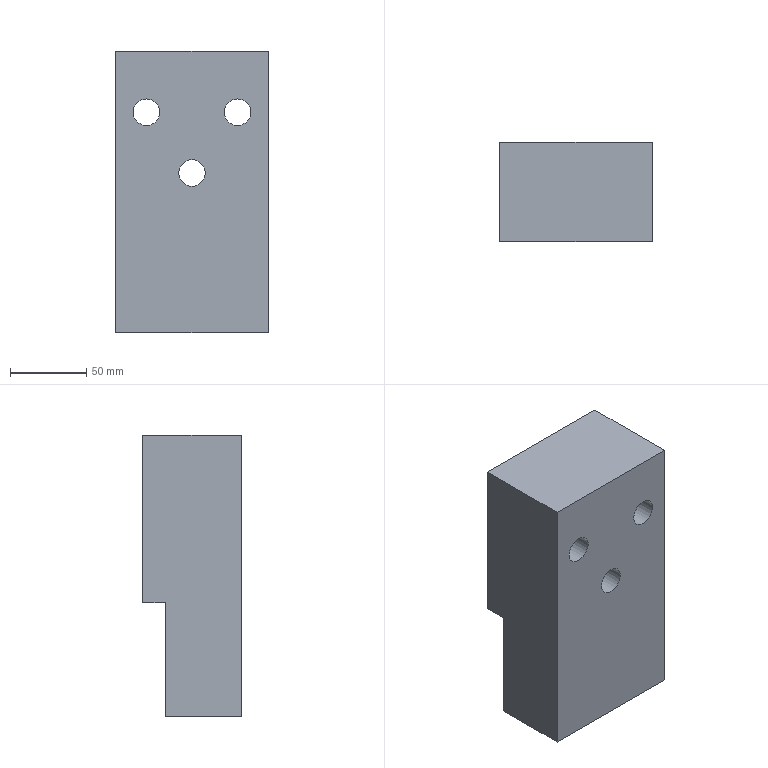Part | NX | features solid 2 | 1 solid | 17 faces | box 100 x 65 x 185 mm | volume 1022834 mm3 | plane 11 | cylinder 6 | commonest cylinder face diameters 17.5 x3 25.5 x3
STEP:
#1=CARTESIAN_POINT('',(452.5,250.,0.));
#2=VERTEX_POINT('',#1);
#3=CARTESIAN_POINT('',(352.5,250.,0.));
#4=VERTEX_POINT('',#3);
#5=CARTESIAN_POINT('',(452.5,250.,0.));
#6=DIRECTION('',(-1.,0.,0.));
#7=VECTOR('',#6,1000.);
#8=LINE('',#5,#7);
#9=EDGE_CURVE('',#2,#4,#8,.T.);
#10=ORIENTED_EDGE('',*,*,#9,.F.);
#11=CARTESIAN_POINT('',(452.5,250.,-75.));
#12=VERTEX_POINT('',#11);
#13=CARTESIAN_POINT('',(452.5,250.,-90.));
#14=DIRECTION('',(0.,0.,1.));
#15=VECTOR('',#14,1000.);
#16=LINE('',#13,#15);
#17=EDGE_CURVE('',#12,#2,#16,.T.);
#18=ORIENTED_EDGE('',*,*,#17,.F.);
#19=CARTESIAN_POINT('',(352.5,250.,-75.));
#20=VERTEX_POINT('',#19);
#21=CARTESIAN_POINT('',(377.5,250.,-75.));
#22=DIRECTION('',(1.,0.,0.));
#23=VECTOR('',#22,1000.);
#24=LINE('',#21,#23);
#25=EDGE_CURVE('',#20,#12,#24,.T.);
#26=ORIENTED_EDGE('',*,*,#25,.F.);
#27=CARTESIAN_POINT('',(352.5,250.,10.));
#28=DIRECTION('',(0.,0.,-1.));
#29=VECTOR('',#28,1000.);
#30=LINE('',#27,#29);
#31=EDGE_CURVE('',#4,#20,#30,.T.);
#32=ORIENTED_EDGE('',*,*,#31,.F.);
#33=EDGE_LOOP('',(#10,#18,#26,#32));
#34=FACE_BOUND('',#33,.T.);
#35=CARTESIAN_POINT('',(377.5,250.,10.));
#36=DIRECTION('',(0.,-1.,0.));
#37=DIRECTION('',(1.,0.,0.));
#38=AXIS2_PLACEMENT_3D('',#35,#36,#37);
#39=PLANE('',#38);
#40=ADVANCED_FACE('',(#34),#39,.F.);
#41=CARTESIAN_POINT('',(452.5,200.,110.));
#42=VERTEX_POINT('',#41);
#43=CARTESIAN_POINT('',(352.5,200.,110.));
#44=VERTEX_POINT('',#43);
#45=CARTESIAN_POINT('',(377.5,200.,110.));
#46=DIRECTION('',(-1.,0.,0.));
#47=VECTOR('',#46,1000.);
#48=LINE('',#45,#47);
#49=EDGE_CURVE('',#42,#44,#48,.T.);
#50=ORIENTED_EDGE('',*,*,#49,.F.);
#51=CARTESIAN_POINT('',(452.5,265.,110.));
#52=VERTEX_POINT('',#51);
#53=CARTESIAN_POINT('',(452.5,250.,110.));
#54=DIRECTION('',(0.,-1.,0.));
#55=VECTOR('',#54,1000.);
#56=LINE('',#53,#55);
#57=EDGE_CURVE('',#52,#42,#56,.T.);
#58=ORIENTED_EDGE('',*,*,#57,.F.);
#59=CARTESIAN_POINT('',(352.5,265.,110.));
#60=VERTEX_POINT('',#59);
#61=CARTESIAN_POINT('',(452.5,265.,110.));
#62=DIRECTION('',(1.,0.,0.));
#63=VECTOR('',#62,1000.);
#64=LINE('',#61,#63);
#65=EDGE_CURVE('',#52,#60,#64,.F.);
#66=ORIENTED_EDGE('',*,*,#65,.T.);
#67=CARTESIAN_POINT('',(352.5,-369.99,110.));
#68=DIRECTION('',(0.,-1.,0.));
#69=VECTOR('',#68,1000.);
#70=LINE('',#67,#69);
#71=EDGE_CURVE('',#60,#44,#70,.T.);
#72=ORIENTED_EDGE('',*,*,#71,.T.);
#73=EDGE_LOOP('',(#50,#58,#66,#72));
#74=FACE_BOUND('',#73,.T.);
#75=CARTESIAN_POINT('',(-1195.,-369.99,110.));
#76=DIRECTION('',(0.,0.,1.));
#77=DIRECTION('',(1.,0.,0.));
#78=AXIS2_PLACEMENT_3D('',#75,#76,#77);
#79=PLANE('',#78);
#80=ADVANCED_FACE('',(#74),#79,.T.);
#81=CARTESIAN_POINT('',(352.5,200.,-75.));
#82=VERTEX_POINT('',#81);
#83=CARTESIAN_POINT('',(352.5,200.,10.));
#84=DIRECTION('',(0.,0.,-1.));
#85=VECTOR('',#84,1000.);
#86=LINE('',#83,#85);
#87=EDGE_CURVE('',#44,#82,#86,.T.);
#88=ORIENTED_EDGE('',*,*,#87,.F.);
#89=ORIENTED_EDGE('',*,*,#71,.F.);
#90=CARTESIAN_POINT('',(352.5,265.,0.));
#91=VERTEX_POINT('',#90);
#92=CARTESIAN_POINT('',(352.5,265.,10.));
#93=DIRECTION('',(0.,0.,1.));
#94=VECTOR('',#93,1000.);
#95=LINE('',#92,#94);
#96=EDGE_CURVE('',#91,#60,#95,.T.);
#97=ORIENTED_EDGE('',*,*,#96,.F.);
#98=CARTESIAN_POINT('',(352.5,250.,0.));
#99=DIRECTION('',(0.,1.,0.));
#100=VECTOR('',#99,1000.);
#101=LINE('',#98,#100);
#102=EDGE_CURVE('',#4,#91,#101,.T.);
#103=ORIENTED_EDGE('',*,*,#102,.F.);
#104=ORIENTED_EDGE('',*,*,#31,.T.);
#105=CARTESIAN_POINT('',(352.5,250.,-75.));
#106=DIRECTION('',(0.,-1.,0.));
#107=VECTOR('',#106,1000.);
#108=LINE('',#105,#107);
#109=EDGE_CURVE('',#20,#82,#108,.T.);
#110=ORIENTED_EDGE('',*,*,#109,.T.);
#111=EDGE_LOOP('',(#88,#89,#97,#103,#104,#110));
#112=FACE_BOUND('',#111,.T.);
#113=CARTESIAN_POINT('',(352.5,250.,10.));
#114=DIRECTION('',(-1.,0.,0.));
#115=DIRECTION('',(0.,0.,1.));
#116=AXIS2_PLACEMENT_3D('',#113,#114,#115);
#117=PLANE('',#116);
#118=ADVANCED_FACE('',(#112),#117,.T.);
#119=CARTESIAN_POINT('',(452.5,200.,-75.));
#120=VERTEX_POINT('',#119);
#121=CARTESIAN_POINT('',(377.5,200.,-75.));
#122=DIRECTION('',(1.,0.,0.));
#123=VECTOR('',#122,1000.);
#124=LINE('',#121,#123);
#125=EDGE_CURVE('',#82,#120,#124,.T.);
#126=ORIENTED_EDGE('',*,*,#125,.F.);
#127=ORIENTED_EDGE('',*,*,#109,.F.);
#128=ORIENTED_EDGE('',*,*,#25,.T.);
#129=CARTESIAN_POINT('',(452.5,250.,-75.));
#130=DIRECTION('',(0.,-1.,0.));
#131=VECTOR('',#130,1000.);
#132=LINE('',#129,#131);
#133=EDGE_CURVE('',#12,#120,#132,.T.);
#134=ORIENTED_EDGE('',*,*,#133,.T.);
#135=EDGE_LOOP('',(#126,#127,#128,#134));
#136=FACE_BOUND('',#135,.T.);
#137=CARTESIAN_POINT('',(377.5,250.,-75.));
#138=DIRECTION('',(0.,0.,-1.));
#139=DIRECTION('',(-1.,0.,0.));
#140=AXIS2_PLACEMENT_3D('',#137,#138,#139);
#141=PLANE('',#140);
#142=ADVANCED_FACE('',(#136),#141,.T.);
#143=CARTESIAN_POINT('',(452.5,200.,-90.));
#144=DIRECTION('',(0.,0.,1.));
#145=VECTOR('',#144,1000.);
#146=LINE('',#143,#145);
#147=EDGE_CURVE('',#120,#42,#146,.T.);
#148=ORIENTED_EDGE('',*,*,#147,.F.);
#149=ORIENTED_EDGE('',*,*,#133,.F.);
#150=ORIENTED_EDGE('',*,*,#17,.T.);
#151=CARTESIAN_POINT('',(452.5,265.,0.));
#152=VERTEX_POINT('',#151);
#153=CARTESIAN_POINT('',(452.5,250.,0.));
#154=DIRECTION('',(0.,1.,0.));
#155=VECTOR('',#154,1000.);
#156=LINE('',#153,#155);
#157=EDGE_CURVE('',#2,#152,#156,.T.);
#158=ORIENTED_EDGE('',*,*,#157,.T.);
#159=CARTESIAN_POINT('',(452.5,265.,10.));
#160=DIRECTION('',(0.,0.,1.));
#161=VECTOR('',#160,1000.);
#162=LINE('',#159,#161);
#163=EDGE_CURVE('',#152,#52,#162,.T.);
#164=ORIENTED_EDGE('',*,*,#163,.T.);
#165=ORIENTED_EDGE('',*,*,#57,.T.);
#166=EDGE_LOOP('',(#148,#149,#150,#158,#164,#165));
#167=FACE_BOUND('',#166,.T.);
#168=CARTESIAN_POINT('',(452.5,250.,-90.));
#169=DIRECTION('',(1.,0.,0.));
#170=DIRECTION('',(0.,0.,-1.));
#171=AXIS2_PLACEMENT_3D('',#168,#169,#170);
#172=PLANE('',#171);
#173=ADVANCED_FACE('',(#167),#172,.T.);
#174=CARTESIAN_POINT('',(402.5,200.,21.25));
#175=VERTEX_POINT('',#174);
#176=CARTESIAN_POINT('',(402.5,200.,30.));
#177=DIRECTION('',(0.,-1.,0.));
#178=DIRECTION('',(0.,0.,-1.));
#179=AXIS2_PLACEMENT_3D('',#176,#177,#178);
#180=CIRCLE('',#179,8.75);
#181=EDGE_CURVE('',#175,#175,#180,.T.);
#182=ORIENTED_EDGE('',*,*,#181,.F.);
#183=EDGE_LOOP('',(#182));
#184=FACE_BOUND('',#183,.T.);
#185=CARTESIAN_POINT('',(432.5,200.,61.25));
#186=VERTEX_POINT('',#185);
#187=CARTESIAN_POINT('',(432.5,200.,70.));
#188=DIRECTION('',(0.,-1.,0.));
#189=DIRECTION('',(0.,0.,-1.));
#190=AXIS2_PLACEMENT_3D('',#187,#188,#189);
#191=CIRCLE('',#190,8.75);
#192=EDGE_CURVE('',#186,#186,#191,.T.);
#193=ORIENTED_EDGE('',*,*,#192,.F.);
#194=EDGE_LOOP('',(#193));
#195=FACE_BOUND('',#194,.T.);
#196=CARTESIAN_POINT('',(372.5,200.,61.25));
#197=VERTEX_POINT('',#196);
#198=CARTESIAN_POINT('',(372.5,200.,70.));
#199=DIRECTION('',(0.,-1.,0.));
#200=DIRECTION('',(0.,0.,-1.));
#201=AXIS2_PLACEMENT_3D('',#198,#199,#200);
#202=CIRCLE('',#201,8.75);
#203=EDGE_CURVE('',#197,#197,#202,.T.);
#204=ORIENTED_EDGE('',*,*,#203,.F.);
#205=EDGE_LOOP('',(#204));
#206=FACE_BOUND('',#205,.T.);
#207=ORIENTED_EDGE('',*,*,#49,.T.);
#208=ORIENTED_EDGE('',*,*,#87,.T.);
#209=ORIENTED_EDGE('',*,*,#125,.T.);
#210=ORIENTED_EDGE('',*,*,#147,.T.);
#211=EDGE_LOOP('',(#207,#208,#209,#210));
#212=FACE_BOUND('',#211,.T.);
#213=CARTESIAN_POINT('',(377.5,200.,10.));
#214=DIRECTION('',(0.,-1.,0.));
#215=DIRECTION('',(1.,0.,0.));
#216=AXIS2_PLACEMENT_3D('',#213,#214,#215);
#217=PLANE('',#216);
#218=ADVANCED_FACE('',(#184,#195,#206,#212),#217,.T.);
#219=CARTESIAN_POINT('',(402.5,265.,17.25));
#220=VERTEX_POINT('',#219);
#221=CARTESIAN_POINT('',(402.5,265.,30.));
#222=DIRECTION('',(0.,-1.,0.));
#223=DIRECTION('',(0.,0.,-1.));
#224=AXIS2_PLACEMENT_3D('',#221,#222,#223);
#225=CIRCLE('',#224,12.75);
#226=EDGE_CURVE('',#220,#220,#225,.T.);
#227=ORIENTED_EDGE('',*,*,#226,.T.);
#228=EDGE_LOOP('',(#227));
#229=FACE_BOUND('',#228,.T.);
#230=CARTESIAN_POINT('',(432.5,265.,57.25));
#231=VERTEX_POINT('',#230);
#232=CARTESIAN_POINT('',(432.5,265.,70.));
#233=DIRECTION('',(0.,-1.,0.));
#234=DIRECTION('',(0.,0.,-1.));
#235=AXIS2_PLACEMENT_3D('',#232,#233,#234);
#236=CIRCLE('',#235,12.75);
#237=EDGE_CURVE('',#231,#231,#236,.T.);
#238=ORIENTED_EDGE('',*,*,#237,.T.);
#239=EDGE_LOOP('',(#238));
#240=FACE_BOUND('',#239,.T.);
#241=CARTESIAN_POINT('',(372.5,265.,57.25));
#242=VERTEX_POINT('',#241);
#243=CARTESIAN_POINT('',(372.5,265.,70.));
#244=DIRECTION('',(0.,-1.,0.));
#245=DIRECTION('',(0.,0.,-1.));
#246=AXIS2_PLACEMENT_3D('',#243,#244,#245);
#247=CIRCLE('',#246,12.75);
#248=EDGE_CURVE('',#242,#242,#247,.T.);
#249=ORIENTED_EDGE('',*,*,#248,.T.);
#250=EDGE_LOOP('',(#249));
#251=FACE_BOUND('',#250,.T.);
#252=ORIENTED_EDGE('',*,*,#65,.F.);
#253=ORIENTED_EDGE('',*,*,#163,.F.);
#254=CARTESIAN_POINT('',(452.5,265.,0.));
#255=DIRECTION('',(-1.,0.,0.));
#256=VECTOR('',#255,1000.);
#257=LINE('',#254,#256);
#258=EDGE_CURVE('',#152,#91,#257,.T.);
#259=ORIENTED_EDGE('',*,*,#258,.T.);
#260=ORIENTED_EDGE('',*,*,#96,.T.);
#261=EDGE_LOOP('',(#252,#253,#259,#260));
#262=FACE_BOUND('',#261,.T.);
#263=CARTESIAN_POINT('',(452.5,265.,10.));
#264=DIRECTION('',(0.,1.,0.));
#265=DIRECTION('',(0.,0.,1.));
#266=AXIS2_PLACEMENT_3D('',#263,#264,#265);
#267=PLANE('',#266);
#268=ADVANCED_FACE('',(#229,#240,#251,#262),#267,.T.);
#269=ORIENTED_EDGE('',*,*,#258,.F.);
#270=ORIENTED_EDGE('',*,*,#157,.F.);
#271=ORIENTED_EDGE('',*,*,#9,.T.);
#272=ORIENTED_EDGE('',*,*,#102,.T.);
#273=EDGE_LOOP('',(#269,#270,#271,#272));
#274=FACE_BOUND('',#273,.T.);
#275=CARTESIAN_POINT('',(452.5,250.,0.));
#276=DIRECTION('',(0.,0.,-1.));
#277=DIRECTION('',(1.,0.,0.));
#278=AXIS2_PLACEMENT_3D('',#275,#276,#277);
#279=PLANE('',#278);
#280=ADVANCED_FACE('',(#274),#279,.T.);
#281=ORIENTED_EDGE('',*,*,#203,.T.);
#282=EDGE_LOOP('',(#281));
#283=FACE_BOUND('',#282,.T.);
#284=CARTESIAN_POINT('',(372.5,240.,61.25));
#285=VERTEX_POINT('',#284);
#286=CARTESIAN_POINT('',(372.5,240.,70.));
#287=DIRECTION('',(0.,-1.,0.));
#288=DIRECTION('',(0.,0.,-1.));
#289=AXIS2_PLACEMENT_3D('',#286,#287,#288);
#290=CIRCLE('',#289,8.75);
#291=EDGE_CURVE('',#285,#285,#290,.T.);
#292=ORIENTED_EDGE('',*,*,#291,.F.);
#293=EDGE_LOOP('',(#292));
#294=FACE_BOUND('',#293,.T.);
#295=CARTESIAN_POINT('',(372.5,165.,70.));
#296=DIRECTION('',(0.,-1.,0.));
#297=DIRECTION('',(0.,0.,-1.));
#298=AXIS2_PLACEMENT_3D('',#295,#296,#297);
#299=CYLINDRICAL_SURFACE('',#298,8.75);
#300=ADVANCED_FACE('',(#283,#294),#299,.F.);
#301=ORIENTED_EDGE('',*,*,#291,.T.);
#302=EDGE_LOOP('',(#301));
#303=FACE_BOUND('',#302,.T.);
#304=CARTESIAN_POINT('',(372.5,240.,57.25));
#305=VERTEX_POINT('',#304);
#306=CARTESIAN_POINT('',(372.5,240.,70.));
#307=DIRECTION('',(0.,-1.,0.));
#308=DIRECTION('',(0.,0.,-1.));
#309=AXIS2_PLACEMENT_3D('',#306,#307,#308);
#310=CIRCLE('',#309,12.75);
#311=EDGE_CURVE('',#305,#305,#310,.T.);
#312=ORIENTED_EDGE('',*,*,#311,.F.);
#313=EDGE_LOOP('',(#312));
#314=FACE_BOUND('',#313,.T.);
#315=CARTESIAN_POINT('',(397.5,240.,70.));
#316=DIRECTION('',(0.,-1.,0.));
#317=DIRECTION('',(0.,0.,-1.));
#318=AXIS2_PLACEMENT_3D('',#315,#316,#317);
#319=PLANE('',#318);
#320=ADVANCED_FACE('',(#303,#314),#319,.F.);
#321=ORIENTED_EDGE('',*,*,#311,.T.);
#322=EDGE_LOOP('',(#321));
#323=FACE_BOUND('',#322,.T.);
#324=ORIENTED_EDGE('',*,*,#248,.F.);
#325=EDGE_LOOP('',(#324));
#326=FACE_BOUND('',#325,.T.);
#327=CARTESIAN_POINT('',(372.5,265.,70.));
#328=DIRECTION('',(0.,-1.,0.));
#329=DIRECTION('',(0.,0.,-1.));
#330=AXIS2_PLACEMENT_3D('',#327,#328,#329);
#331=CYLINDRICAL_SURFACE('',#330,12.75);
#332=ADVANCED_FACE('',(#323,#326),#331,.F.);
#333=ORIENTED_EDGE('',*,*,#192,.T.);
#334=EDGE_LOOP('',(#333));
#335=FACE_BOUND('',#334,.T.);
#336=CARTESIAN_POINT('',(432.5,240.,61.25));
#337=VERTEX_POINT('',#336);
#338=CARTESIAN_POINT('',(432.5,240.,70.));
#339=DIRECTION('',(0.,-1.,0.));
#340=DIRECTION('',(0.,0.,-1.));
#341=AXIS2_PLACEMENT_3D('',#338,#339,#340);
#342=CIRCLE('',#341,8.75);
#343=EDGE_CURVE('',#337,#337,#342,.T.);
#344=ORIENTED_EDGE('',*,*,#343,.F.);
#345=EDGE_LOOP('',(#344));
#346=FACE_BOUND('',#345,.T.);
#347=CARTESIAN_POINT('',(432.5,165.,70.));
#348=DIRECTION('',(0.,-1.,0.));
#349=DIRECTION('',(0.,0.,-1.));
#350=AXIS2_PLACEMENT_3D('',#347,#348,#349);
#351=CYLINDRICAL_SURFACE('',#350,8.75);
#352=ADVANCED_FACE('',(#335,#346),#351,.F.);
#353=ORIENTED_EDGE('',*,*,#343,.T.);
#354=EDGE_LOOP('',(#353));
#355=FACE_BOUND('',#354,.T.);
#356=CARTESIAN_POINT('',(432.5,240.,57.25));
#357=VERTEX_POINT('',#356);
#358=CARTESIAN_POINT('',(432.5,240.,70.));
#359=DIRECTION('',(0.,-1.,0.));
#360=DIRECTION('',(0.,0.,-1.));
#361=AXIS2_PLACEMENT_3D('',#358,#359,#360);
#362=CIRCLE('',#361,12.75);
#363=EDGE_CURVE('',#357,#357,#362,.T.);
#364=ORIENTED_EDGE('',*,*,#363,.F.);
#365=EDGE_LOOP('',(#364));
#366=FACE_BOUND('',#365,.T.);
#367=CARTESIAN_POINT('',(432.5,240.,70.));
#368=DIRECTION('',(0.,-1.,0.));
#369=DIRECTION('',(0.,0.,-1.));
#370=AXIS2_PLACEMENT_3D('',#367,#368,#369);
#371=PLANE('',#370);
#372=ADVANCED_FACE('',(#355,#366),#371,.F.);
#373=ORIENTED_EDGE('',*,*,#363,.T.);
#374=EDGE_LOOP('',(#373));
#375=FACE_BOUND('',#374,.T.);
#376=ORIENTED_EDGE('',*,*,#237,.F.);
#377=EDGE_LOOP('',(#376));
#378=FACE_BOUND('',#377,.T.);
#379=CARTESIAN_POINT('',(432.5,265.,70.));
#380=DIRECTION('',(0.,-1.,0.));
#381=DIRECTION('',(0.,0.,-1.));
#382=AXIS2_PLACEMENT_3D('',#379,#380,#381);
#383=CYLINDRICAL_SURFACE('',#382,12.75);
#384=ADVANCED_FACE('',(#375,#378),#383,.F.);
#385=ORIENTED_EDGE('',*,*,#181,.T.);
#386=EDGE_LOOP('',(#385));
#387=FACE_BOUND('',#386,.T.);
#388=CARTESIAN_POINT('',(402.5,240.,21.25));
#389=VERTEX_POINT('',#388);
#390=CARTESIAN_POINT('',(402.5,240.,30.));
#391=DIRECTION('',(0.,-1.,0.));
#392=DIRECTION('',(0.,0.,-1.));
#393=AXIS2_PLACEMENT_3D('',#390,#391,#392);
#394=CIRCLE('',#393,8.75);
#395=EDGE_CURVE('',#389,#389,#394,.T.);
#396=ORIENTED_EDGE('',*,*,#395,.F.);
#397=EDGE_LOOP('',(#396));
#398=FACE_BOUND('',#397,.T.);
#399=CARTESIAN_POINT('',(402.5,165.,30.));
#400=DIRECTION('',(0.,-1.,0.));
#401=DIRECTION('',(0.,0.,-1.));
#402=AXIS2_PLACEMENT_3D('',#399,#400,#401);
#403=CYLINDRICAL_SURFACE('',#402,8.75);
#404=ADVANCED_FACE('',(#387,#398),#403,.F.);
#405=ORIENTED_EDGE('',*,*,#395,.T.);
#406=EDGE_LOOP('',(#405));
#407=FACE_BOUND('',#406,.T.);
#408=CARTESIAN_POINT('',(402.5,240.,17.25));
#409=VERTEX_POINT('',#408);
#410=CARTESIAN_POINT('',(402.5,240.,30.));
#411=DIRECTION('',(0.,-1.,0.));
#412=DIRECTION('',(0.,0.,-1.));
#413=AXIS2_PLACEMENT_3D('',#410,#411,#412);
#414=CIRCLE('',#413,12.75);
#415=EDGE_CURVE('',#409,#409,#414,.T.);
#416=ORIENTED_EDGE('',*,*,#415,.F.);
#417=EDGE_LOOP('',(#416));
#418=FACE_BOUND('',#417,.T.);
#419=CARTESIAN_POINT('',(402.5,240.,30.));
#420=DIRECTION('',(0.,-1.,0.));
#421=DIRECTION('',(0.,0.,-1.));
#422=AXIS2_PLACEMENT_3D('',#419,#420,#421);
#423=PLANE('',#422);
#424=ADVANCED_FACE('',(#407,#418),#423,.F.);
#425=ORIENTED_EDGE('',*,*,#415,.T.);
#426=EDGE_LOOP('',(#425));
#427=FACE_BOUND('',#426,.T.);
#428=ORIENTED_EDGE('',*,*,#226,.F.);
#429=EDGE_LOOP('',(#428));
#430=FACE_BOUND('',#429,.T.);
#431=CARTESIAN_POINT('',(402.5,265.,30.));
#432=DIRECTION('',(0.,-1.,0.));
#433=DIRECTION('',(0.,0.,-1.));
#434=AXIS2_PLACEMENT_3D('',#431,#432,#433);
#435=CYLINDRICAL_SURFACE('',#434,12.75);
#436=ADVANCED_FACE('',(#427,#430),#435,.F.);
#437=CLOSED_SHELL('',(#40,#80,#118,#142,#173,#218,#268,#280,#300,#320,#332,#352,#372,#384,#404,#424,#436));
#438=MANIFOLD_SOLID_BREP('',#437);
#439=(LENGTH_UNIT()NAMED_UNIT(*)SI_UNIT(.MILLI.,.METRE.));
#440=UNCERTAINTY_MEASURE_WITH_UNIT(LENGTH_MEASURE(0.00001),#439,'','');
#441=(NAMED_UNIT(*)PLANE_ANGLE_UNIT()SI_UNIT($,.RADIAN.));
#442=(NAMED_UNIT(*)SI_UNIT($,.STERADIAN.)SOLID_ANGLE_UNIT());
#443=(GEOMETRIC_REPRESENTATION_CONTEXT(3)GLOBAL_UNCERTAINTY_ASSIGNED_CONTEXT((#440))GLOBAL_UNIT_ASSIGNED_CONTEXT((#439,#441,#442))REPRESENTATION_CONTEXT('',''));
#444=ADVANCED_BREP_SHAPE_REPRESENTATION('',(#438),#443);